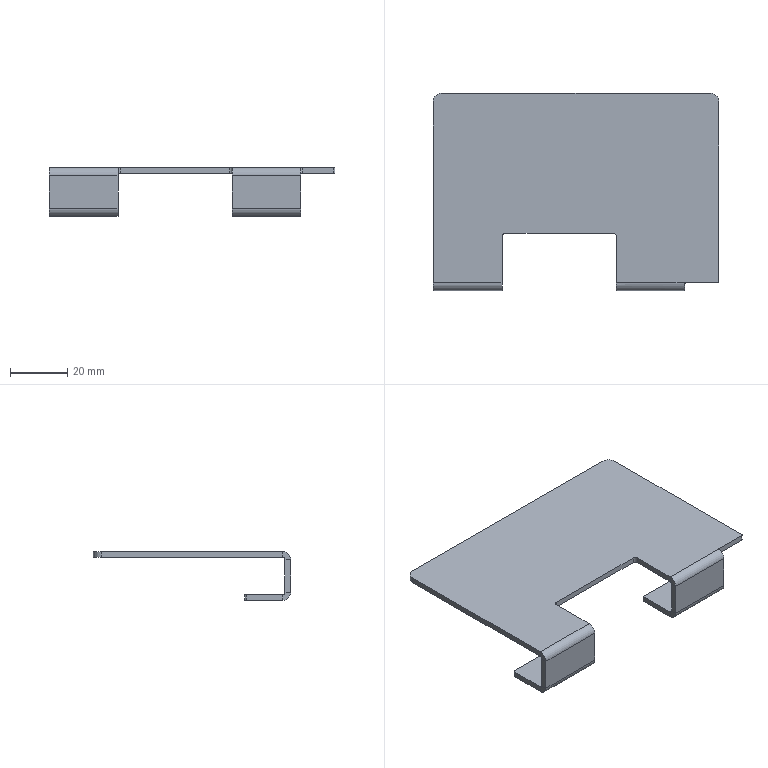Part | STEP file | H_ND25042-01-JG-001-BJ | 1 solid | 50 faces | box 100 x 69 x 17 mm | volume 14768 mm3 | plane 34 | cylinder 16 | commonest cylinder face diameters 1 x4 1.473 x4 5.473 x4 2 x2 6 x2